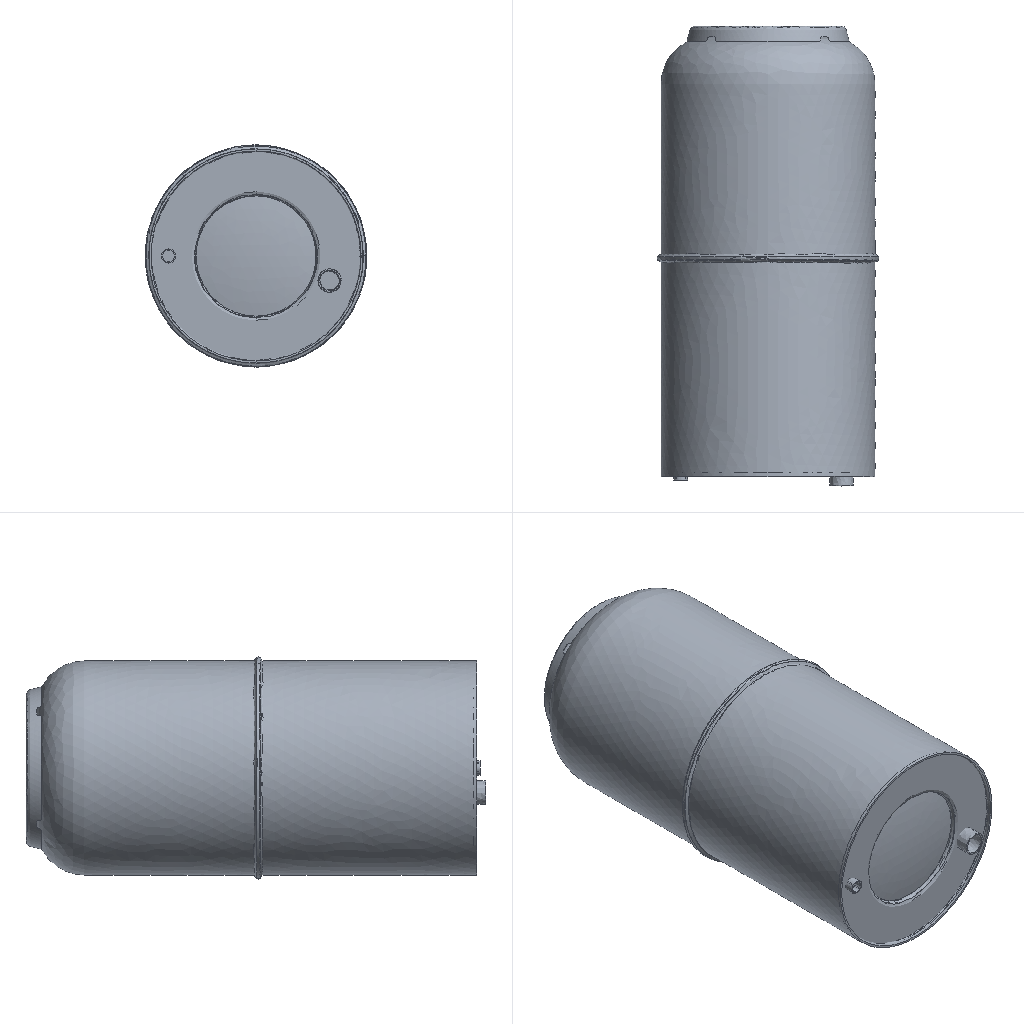Simulation study | ansys workbench
Ansys APDL input file, long lists of numbers shortened:
/batch
/config,noeldb,1     ! force off writing results to database
*get,_wallstrt,active,,time,wall
! ANSYS input file written by Workbench version 2024 R2
! File used for geometry attach:
/title,___--___ (B5)
! ****** Begin Custom Load Command Snippet ******
/COM, ACT Extensions:
/COM,     LSDYNA, 2024.2
/COM,/COM,     ANSYSMotion, 2024.2
/COM,
! ****** End   Custom Load Command Snippet ******
/com,--- Data in consistent NMM units. See Solving Units in the help system for more information.
/units,MPA
/nopr
/wb,file,start              !  signify a WB generated input file
/prep7
! Turn off shape checking because checks already performed inside WB mesher.
! See help system for more information.
SHPP,OFF,,NOWARN
/nolist
etcon,set             ! allow ANSYS to choose best KEYOP's for 180x elements, resets any applicable keyopt to MAPDL defaults
/com,*********** Nodes for the whole assembly ***********
nblock,3,,111691
(1i9,3e20.9e3)
        1    -1.335648785E-14     5.482400000E+01     5.453200000E+01
! (101537 more lines like these left out)
-1
/wb,elem,start            !  set before creation of elements
/com,*********** Elements for Body 1 'Z_ASM_35_ASM|PRT0001_21|PRT0001_21' ***********
et,1,291
eblock,19,solid,,41186
(19i9)
        1        1        1        1        0        0        0        0       10        0        1     1222     3979     1223     4152    24811    24824    24807    24813
! (82371 more lines like these left out)
-1
/com,*********** Elements for Body 2 'Z_ASM_35_ASM|20X14_1|20X14_1' ***********
et,2,291
eblock,19,solid,,1068
(19i9)
        2        2        2        2        0        0        0        0       10        0    41187    81453    81537    81589    81690    82196    82698    82198    82203
! (2135 more lines like these left out)
-1
/com,*********** Elements for Body 3 'Z_ASM_35_ASM|DN15-1_1|DN15-1_1' ***********
et,3,291
eblock,19,solid,,2313
(19i9)
        3        3        3        3        0        0        0        0       10        0    42255    84534    84608    84567    84568    88980    89086    88973    88974
! (4625 more lines like these left out)
-1
/com,*********** Elements for Body 4 'Z_ASM_35_ASM|5_22|5_22' ***********
et,4,291
eblock,19,solid,,5247
(19i9)
        4        4        4        4        0        0        0        0       10        0    44568    89485    90565    90603    90604    92828    99020    92829    92830
! (10493 more lines like these left out)
-1
/com,*********** Elements for Body 5 'Z_ASM_35_ASM|DN6_35_2|DN6_35_2' ***********
et,5,279
eblock,19,solid,,156
(19i9)
        5        5        5        5        0        0        0        0       20        0    49815   100606   100658   100657   100607   100623   100672   100671   100624
! (311 more lines like these left out)
-1
/wb,elem,end               !  done creating elements
/com,*********** Send User Defined Coordinate System(s) ***********
csys,0
toffst,273.15,      ! Temperature offset from absolute zero
/wb,mat,start              !  starting to send materials
/com,*********** Send Materials ***********
Temperature = 'TEMP' ! Temperature
MP,DENS,1,7.75e-09,	! tonne mm^-3
MP,ALPX,1,1.7e-05,	! C^-1
MP,C,1,480000000,	! mm^2 s^-2 C^-1
MP,KXX,1,15.1,	! tonne mm s^-3 C^-1
MP,RSVX,1,0.00077,	! ohm mm
MP,EX,1,193000,	! tonne s^-2 mm^-1
MP,NUXY,1,0.31,
MP,MURX,1,1,
Temperature = 'TEMP' ! Temperature
MP,DENS,2,7.75e-09,	! tonne mm^-3
MP,ALPX,2,1.7e-05,	! C^-1
MP,C,2,480000000,	! mm^2 s^-2 C^-1
MP,KXX,2,15.1,	! tonne mm s^-3 C^-1
MP,RSVX,2,0.00077,	! ohm mm
MP,EX,2,193000,	! tonne s^-2 mm^-1
MP,NUXY,2,0.31,
MP,MURX,2,1,
Temperature = 'TEMP' ! Temperature
MP,DENS,3,7.75e-09,	! tonne mm^-3
MP,ALPX,3,1.7e-05,	! C^-1
MP,C,3,480000000,	! mm^2 s^-2 C^-1
MP,KXX,3,15.1,	! tonne mm s^-3 C^-1
MP,RSVX,3,0.00077,	! ohm mm
MP,EX,3,193000,	! tonne s^-2 mm^-1
MP,NUXY,3,0.31,
MP,MURX,3,1,
Temperature = 'TEMP' ! Temperature
MP,DENS,4,7.75e-09,	! tonne mm^-3
MP,ALPX,4,1.7e-05,	! C^-1
MP,C,4,480000000,	! mm^2 s^-2 C^-1
MP,KXX,4,15.1,	! tonne mm s^-3 C^-1
MP,RSVX,4,0.00077,	! ohm mm
MP,EX,4,193000,	! tonne s^-2 mm^-1
MP,NUXY,4,0.31,
MP,MURX,4,1,
Temperature = 'TEMP' ! Temperature
MP,DENS,5,7.75e-09,	! tonne mm^-3
MP,ALPX,5,1.7e-05,	! C^-1
MP,C,5,480000000,	! mm^2 s^-2 C^-1
MP,KXX,5,15.1,	! tonne mm s^-3 C^-1
MP,RSVX,5,0.00077,	! ohm mm
MP,EX,5,193000,	! tonne s^-2 mm^-1
MP,NUXY,5,0.31,
MP,MURX,5,1,
/wb,mat,end                !  done sending materials
!************************* Model Summary ********************
!Z_ASM_35_ASM|PRT0001_21|PRT0001_21,	304é¢,	matid,	1
!Z_ASM_35_ASM|20X14_1|20X14_1,	304é¢,	matid,	2
!Z_ASM_35_ASM|DN15-1_1|DN15-1_1,	304é¢,	matid,	3
!Z_ASM_35_ASM|5_22|5_22,	304é¢,	matid,	4
!Z_ASM_35_ASM|DN6_35_2|DN6_35_2,	304é¢,	matid,	5
!************************* End Model Summary ********************
! get the diagonal of the bounding box. Needed later for other things
*get,_xmin,node,,mnloc,x
*get,_ymin,node,,mnloc,y
*get,_zmin,node,,mnloc,z
*get,_xmax,node,,mxloc,x
*get,_ymax,node,,mxloc,y
*get,_zmax,node,,mxloc,z
_ASMDIAG=(_xmax-_xmin)*(_xmax-_xmin)+(_ymax-_ymin)*(_ymax-_ymin)+(_zmax-_zmin)*(_zmax-_zmin)
_ASMDIAG=SQRT(_ASMDIAG)
/wb,contact,start          !  starting to send contact
/com,*********** Create Contact "½Ó´¥ÇøÓò" ***********
/com,            Real Constant Set For Above Contact Is 7 & 6
*set,tid,7
*set,cid,6
r,tid
r,cid
et,tid,170
et,cid,174
eblock,10,,,49
(15i9)
    83777        7        7        7        0     1755     1754     2895     2895    29205    29208     2895    29214
! (48 more lines like these left out)
-1
eblock,10,,,49
(15i9)
    83826        6        6        6        0     1755     1754     2895     2895    29205    29208     2895    29214
! (48 more lines like these left out)
-1
eblock,10,,,56
(15i9)
    83875        6        7        6        0    81461    81469    81463    81463    82264    82276    81463    82263
! (55 more lines like these left out)
-1
eblock,10,,,56
(15i9)
    83931        7        6        7        0    81461    81469    81463    81463    82264    82276    81463    82263
! (55 more lines like these left out)
-1
keyo,cid,8,2               ! auto create asymmetric contact (from Program Controlled setting)
keyo,cid,10,0              ! adjust contact stiffness each NR iteration (from Program Controlled setting)
keyo,cid,12,5              ! bonded always
keyo,cid,18,1              ! small sliding turned on by application
keyo,cid,2,0               ! augmented Lagrange (from Program Controlled setting)
keyo,cid,4,0               ! on Gauss point (from Program Controlled setting)
keyo,cid,9,1               ! ignore initial gaps/penetration
keyo,cid,7,0               ! No Prediction
rmod,tid,3,10.      ! FKN
rmod,tid,5,0.       ! ICONT
rmod,tid,6,0.       ! PINB
rmod,tid,10,0.      ! CNOF
rmod,tid,12,0.      ! FKT
rmod,tid,36,39      ! WB DSID
rmod,cid,3,10.      ! FKN
rmod,cid,5,0.       ! ICONT
rmod,cid,6,0.       ! PINB
rmod,cid,10,0.      ! CNOF
rmod,cid,12,0.      ! FKT
rmod,cid,36,39      ! WB DSID
*set,_maxkxx,151000.
rmod,cid,14,_maxkxx/_ASMDIAG         ! TCC, Divide by Length since Traction Based
rmod,tid,14,_maxkxx/_ASMDIAG      ! TCC, Divide by Length since Traction Based
keyo,cid,1,2     ! Pure thermal contact
/com,*********** Create Contact "½Ó´¥ÇøÓò 2" ***********
/com,            Real Constant Set For Above Contact Is 9 & 8
*set,tid,9
*set,cid,8
r,tid
r,cid
et,tid,170
et,cid,174
eblock,10,,,17
(15i9)
    83987        9        9        9        0    12338    12368    12369    12369    79729    79959    12369    79730
! (16 more lines like these left out)
-1
eblock,10,,,17
(15i9)
    84004        8        8        8        0    12338    12368    12369    12369    79729    79959    12369    79730
! (16 more lines like these left out)
-1
eblock,10,,,28
(15i9)
    84021        8        9        8        0    83837    84450    84442    84442    86125    88506    84442    86123
! (27 more lines like these left out)
-1
eblock,10,,,28
(15i9)
    84049        9        8        9        0    83837    84450    84442    84442    86125    88506    84442    86123
! (27 more lines like these left out)
-1
keyo,cid,8,2               ! auto create asymmetric contact (from Program Controlled setting)
keyo,cid,10,0              ! adjust contact stiffness each NR iteration (from Program Controlled setting)
keyo,cid,12,5              ! bonded always
keyo,cid,18,1              ! small sliding turned on by application
keyo,cid,2,0               ! augmented Lagrange (from Program Controlled setting)
keyo,cid,4,0               ! on Gauss point (from Program Controlled setting)
keyo,cid,9,1               ! ignore initial gaps/penetration
keyo,cid,7,0               ! No Prediction
rmod,tid,3,10.      ! FKN
rmod,tid,5,0.       ! ICONT
rmod,tid,6,0.       ! PINB
rmod,tid,10,0.      ! CNOF
rmod,tid,12,0.      ! FKT
rmod,tid,36,42      ! WB DSID
rmod,cid,3,10.      ! FKN
rmod,cid,5,0.       ! ICONT
rmod,cid,6,0.       ! PINB
rmod,cid,10,0.      ! CNOF
rmod,cid,12,0.      ! FKT
rmod,cid,36,42      ! WB DSID
*set,_maxkxx,151000.
rmod,cid,14,_maxkxx/_ASMDIAG         ! TCC, Divide by Length since Traction Based
rmod,tid,14,_maxkxx/_ASMDIAG      ! TCC, Divide by Length since Traction Based
keyo,cid,1,2     ! Pure thermal contact
/com,*********** Create Contact "½Ó´¥ÇøÓò 3" ***********
/com,            Real Constant Set For Above Contact Is 11 & 10
*set,tid,11
*set,cid,10
r,tid
r,cid
et,tid,170
et,cid,174
eblock,10,,,130
(15i9)
    84077       11       11       11        0      228      227      230      230    15322    15323      230    15328
! (129 more lines like these left out)
-1
eblock,10,,,130
(15i9)
    84207       10       10       10        0      228      227      230      230    15322    15323      230    15328
! (129 more lines like these left out)
-1
eblock,10,,,144
(15i9)
    84337       10       11       10        0    89950    89949    89947    89947    96181    96173    89947    96174
! (143 more lines like these left out)
-1
eblock,10,,,144
(15i9)
    84481       11       10       11        0    89950    89949    89947    89947    96181    96173    89947    96174
! (143 more lines like these left out)
-1
keyo,cid,8,2               ! auto create asymmetric contact (from Program Controlled setting)
keyo,cid,10,0              ! adjust contact stiffness each NR iteration (from Program Controlled setting)
keyo,cid,12,5              ! bonded always
keyo,cid,18,1              ! small sliding turned on by application
keyo,cid,2,0               ! augmented Lagrange (from Program Controlled setting)
keyo,cid,4,0               ! on Gauss point (from Program Controlled setting)
keyo,cid,9,1               ! ignore initial gaps/penetration
keyo,cid,7,0               ! No Prediction
rmod,tid,3,10.      ! FKN
rmod,tid,5,0.       ! ICONT
rmod,tid,6,0.       ! PINB
rmod,tid,10,0.      ! CNOF
rmod,tid,12,0.      ! FKT
rmod,tid,36,45      ! WB DSID
rmod,cid,3,10.      ! FKN
rmod,cid,5,0.       ! ICONT
rmod,cid,6,0.       ! PINB
rmod,cid,10,0.      ! CNOF
rmod,cid,12,0.      ! FKT
rmod,cid,36,45      ! WB DSID
*set,_maxkxx,151000.
rmod,cid,14,_maxkxx/_ASMDIAG         ! TCC, Divide by Length since Traction Based
rmod,tid,14,_maxkxx/_ASMDIAG      ! TCC, Divide by Length since Traction Based
keyo,cid,1,2     ! Pure thermal contact
/com,*********** Create Contact "½Ó´¥ÇøÓò 4" ***********
/com,            Real Constant Set For Above Contact Is 13 & 12
*set,tid,13
*set,cid,12
r,tid
r,cid
et,tid,170
et,cid,174
eblock,10,,,28
(15i9)
    84625       13       13       13        0    12555      866    13117    13117    21080    21082    13117    80661
! (27 more lines like these left out)
-1
eblock,10,,,28
(15i9)
    84653       12       12       12        0    12555      866    13117    13117    21080    21082    13117    80661
! (27 more lines like these left out)
-1
eblock,10,,,39
(15i9)
    84681       12       13       12        0   100452   100445   100453   100453   100876   100877   100453   100894
! (38 more lines like these left out)
-1
eblock,10,,,39
(15i9)
    84720       13       12       13        0   100452   100445   100453   100453   100876   100877   100453   100894
! (38 more lines like these left out)
-1
keyo,cid,8,2               ! auto create asymmetric contact (from Program Controlled setting)
keyo,cid,10,0              ! adjust contact stiffness each NR iteration (from Program Controlled setting)
keyo,cid,12,5              ! bonded always
keyo,cid,18,1              ! small sliding turned on by application
keyo,cid,2,0               ! augmented Lagrange (from Program Controlled setting)
keyo,cid,4,0               ! on Gauss point (from Program Controlled setting)
keyo,cid,9,1               ! ignore initial gaps/penetration
keyo,cid,7,0               ! No Prediction
rmod,tid,3,10.      ! FKN
rmod,tid,5,0.       ! ICONT
rmod,tid,6,0.       ! PINB
rmod,tid,10,0.      ! CNOF
rmod,tid,12,0.      ! FKT
rmod,tid,36,48      ! WB DSID
rmod,cid,3,10.      ! FKN
rmod,cid,5,0.       ! ICONT
rmod,cid,6,0.       ! PINB
rmod,cid,10,0.      ! CNOF
rmod,cid,12,0.      ! FKT
rmod,cid,36,48      ! WB DSID
*set,_maxkxx,151000.
rmod,cid,14,_maxkxx/_ASMDIAG         ! TCC, Divide by Length since Traction Based
rmod,tid,14,_maxkxx/_ASMDIAG      ! TCC, Divide by Length since Traction Based
keyo,cid,1,2     ! Pure thermal contact
/com,*********** Create Contact "½Ó´¥ÇøÓò 5" ***********
/com,            Real Constant Set For Above Contact Is 15 & 14
*set,tid,15
*set,cid,14
r,tid
r,cid
et,tid,170
et,cid,174
eblock,10,,,74
(15i9)
    84759       15       15       15        0    81598    81483    81466    81466    82390    82290    81466    82291
! (73 more lines like these left out)
-1
eblock,10,,,74
(15i9)
    84833       14       14       14        0    81598    81483    81466    81466    82390    82290    81466    82291
! (73 more lines like these left out)
-1
eblock,10,,,73
(15i9)
    84907       14       15       14        0    83682    84442    84599    84599    85203    88507    84599    85205
! (72 more lines like these left out)
-1
eblock,10,,,73
(15i9)
    84980       15       14       15        0    83682    84442    84599    84599    85203    88507    84599    85205
! (72 more lines like these left out)
-1
keyo,cid,8,2               ! auto create asymmetric contact (from Program Controlled setting)
keyo,cid,10,0              ! adjust contact stiffness each NR iteration (from Program Controlled setting)
keyo,cid,12,5              ! bonded always
keyo,cid,18,1              ! small sliding turned on by application
keyo,cid,2,0               ! augmented Lagrange (from Program Controlled setting)
keyo,cid,4,0               ! on Gauss point (from Program Controlled setting)
keyo,cid,9,1               ! ignore initial gaps/penetration
keyo,cid,7,0               ! No Prediction
rmod,tid,3,10.      ! FKN
rmod,tid,5,0.       ! ICONT
rmod,tid,6,0.       ! PINB
rmod,tid,10,0.      ! CNOF
rmod,tid,12,0.      ! FKT
rmod,tid,36,51      ! WB DSID
rmod,cid,3,10.      ! FKN
rmod,cid,5,0.       ! ICONT
rmod,cid,6,0.       ! PINB
rmod,cid,10,0.      ! CNOF
rmod,cid,12,0.      ! FKT
rmod,cid,36,51      ! WB DSID
*set,_maxkxx,151000.
rmod,cid,14,_maxkxx/_ASMDIAG         ! TCC, Divide by Length since Traction Based
rmod,tid,14,_maxkxx/_ASMDIAG      ! TCC, Divide by Length since Traction Based
keyo,cid,1,2     ! Pure thermal contact
nsel,all
esel,all
/wb,contact,end            !  done creating contacts
/golist
/wb,load,start             !  starting to send loads
/com,*********** Define Temperature Constraint ***********
CMBLOCK,_CM65   ,NODE,    10039
(8i10)
        20        26        27        28        29        30        31        32
! (1254 more lines like these left out)
fcum,add                   ! add nodal forces up (needed in case have loads on the same edge,vertex)
fcum                       ! reset default on fcum command since done sending WB F loads
/com,*********** Create "______" ***********
et,16,152
eblock,10,,,9987
(15i9)
    85053       16       16       16        0    13119      808      720      720    20542    20006      720    20007
! (9986 more lines like these left out)
-1
esel,s,type,,16
keyop,16,8,4
keyop,16,13,0
/com,*********** Create "_______________" ***********
et,17,152
eblock,10,,,3467
(15i9)
    95040       17       17       17        0     1812     1811     6089     6089    29595    29600     6089    29605
! (3466 more lines like these left out)
-1
esel,s,type,,17
keyop,17,8,4
keyop,17,13,0
esel,all
/com,***************** Define Uniform Initial temperature ***************
tunif,96.
/gst,on,on
fini
*get,_numnode,node,0,count
*get,_numelem,elem,0,count
*get, _MAXELEMNUM, elem, 0, NUM, MAX
*get, _MAXNODENUM, node, 0, NUM, MAX
*get, _MAXELEMTYPE, etyp, 0, NUM, MAX
*get, _MAXREALCONST, rcon, 0, NUM, MAX
/go
/wb,load,end               !  done creating loads
/com,--- Number of total nodes = %_numnode%
/com,--- Number of contact elements = 14730
/com,--- Number of spring elements = 0
/com,--- Number of bearing elements = 0
/com,--- Number of solid elements = 49970
/com,--- Number of condensed parts = 0
/com,--- Number of total elements = %_numelem%
*get,_wallbsol,active,,time,wall
/com,****************************************************************************
/com,*************************    SOLUTION       ********************************
/com,****************************************************************************
/solu
antype,4                   ! transient analysis
kbc,1                      ! stepped BC's
!eqsl,sparse               ! using sparse solver which is default so no eqsl command needed
cntr,print,1               ! print out contact info and also make no initial contact an error
rescontrol,,none                 ! Do not keep any restart files
dmpoption,emat,no             ! Don't combine emat file for DANSYS
dmpoption,esav,no             ! Don't combine esav file for DANSYS
thopt,quasi,5.e-002
nlhist,nsol,MAX_TEMP,temp,max
nlhist,nsol,MIN_TEMP,temp,min
/com,********* Initial Time Increment Check And Fourier Modulus *********
/com, Specified Initial Time Increment: 0.001
/com, Estimated Increment Needed, le*le/alpha, Body 1: 1.098
/com, Estimated Increment Needed, le*le/alpha, Body 2: 0.341
/com, Estimated Increment Needed, le*le/alpha, Body 3: 0.3572
/com, Estimated Increment Needed, le*le/alpha, Body 4: 0.3372
/com, Estimated Increment Needed, le*le/alpha, Body 5: 0.3608
/com,****************************************************
/com,******************* SOLVE FOR LS 1 OF 3 ****************
d,_CM65,temp,96.
esel,s,type,,16
nsle
sf,all,conv,2.8e-005,20.
esel,s,type,,17
nsle
sf,all,conv,1.e-007,22.
nsel,all
esel,all
/nopr
/gopr
autots,on
nsub,100,1000,10
time,0.1
timint,on                  ! Turn on time integration effects
outres,erase
outres,all,none
outres,nsol,all
outres,rsol,all
outres,eangl,all
outres,veng,all
outres,fflux,all,
outres,cont,all,
/nopr
esel,s,type,,16
esel,a,type,,17
cm,_elmisc,elem
esel,all
/gopr
outres,misc,all,_elmisc
cnvtol,heat,,1.e-003,,1.e-003 ! Program Controlled. Set MINREF equivalent of 1e-6 Watts
! *********** WB SOLVE COMMAND ***********
! check interactive state
*get,ANSINTER_,active,,int
*if,ANSINTER_,ne,0,then
/eof
*endif
solve
/com *************** Write FE CONNECTORS *********
CEWRITE,file,ce,,INTE
/com,****************************************************
/com,*************** FINISHED SOLVE FOR LS 1 *************
/com,****************************************************
/com,******************* SOLVE FOR LS 2 OF 3 ****************
ddel,_CM65,temp
/nopr
/gopr
autots,on
nsub,100,1000,10
time,43200.
timint,on                  ! Turn on time integration effects
outres,erase
outres,all,none
outres,nsol,all
outres,rsol,all
outres,eangl,all
outres,veng,all
outres,fflux,all,
outres,cont,all,
outres,misc,all,_elmisc
cnvtol,heat,,1.e-003,,1.e-003 ! Program Controlled. Set MINREF equivalent of 1e-6 Watts
solve
/com,****************************************************
/com,*************** FINISHED SOLVE FOR LS 2 *************
/com,****************************************************
/com,******************* SOLVE FOR LS 3 OF 3 ****************
/nopr
/gopr
autots,on
nsub,100,1000,10
time,86400.
timint,on                  ! Turn on time integration effects
outres,erase
outres,all,none
outres,nsol,all
outres,rsol,all
outres,eangl,all
outres,veng,all
outres,fflux,all,
outres,cont,all,
outres,misc,all,_elmisc
cnvtol,heat,,1.e-003,,1.e-003 ! Program Controlled. Set MINREF equivalent of 1e-6 Watts
solve
/com,****************************************************
/com,*************** FINISHED SOLVE FOR LS 3 *************
*get,_wallasol,active,,time,wall
/post1
xmlo,ENCODING,ISO-8859-1
xmlo,parm
/xml,parm,xml
fini
/gopr
*get,_walldone,active,,time,wall
_preptime=(_wallbsol-_wallstrt)*3600
_solvtime=(_wallasol-_wallbsol)*3600
_posttime=(_walldone-_wallasol)*3600
_totaltim=(_walldone-_wallstrt)*3600
*get,_dlbratio,active,0,solu,dlbr
*get,_combtime,active,0,solu,comb
*get,_ssmode,active,0,solu,ssmm
*get,_ndofs,active,0,solu,ndof
/fclean				!clean distributed files
/com,--- Total number of nodes = %_numnode%
/com,--- Total number of elements = %_numelem%
/com,--- Element load balance ratio = %_dlbratio%
/com,--- Time to combine distributed files = %_combtime%
/com,--- Sparse memory mode = %_ssmode%
/com,--- Number of DOF = %_ndofs%
/wb,file,end               ! done with WB generated input